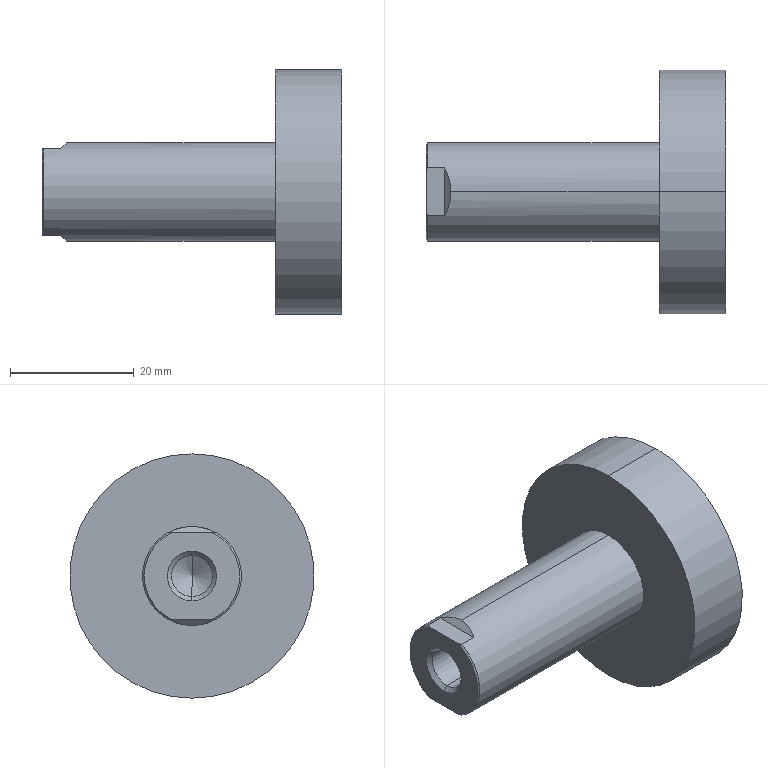Part | SolidWorks | features BaseBody 1 | 1 solid | 19 faces | box 48.5 x 39.5 x 39.5 mm | volume 20251 mm3 | plane 7 | cylinder 6 | cone 6 | commonest cylinder face diameters 6.647 x2 16 x2 39.5 x2
STEP:
#1=CARTESIAN_POINT('',(30.7,0.,8.));
#2=VERTEX_POINT('',#1);
#3=CARTESIAN_POINT('',(30.7,0.,-8.));
#4=VERTEX_POINT('',#3);
#5=CARTESIAN_POINT('',(30.7,0.,0.));
#6=DIRECTION('',(-1.,0.,0.));
#7=DIRECTION('',(0.,0.,1.));
#8=AXIS2_PLACEMENT_3D('',#5,#6,#7);
#9=CIRCLE('',#8,8.);
#10=EDGE_CURVE('',#2,#4,#9,.T.);
#11=ORIENTED_EDGE('',*,*,#10,.T.);
#12=CARTESIAN_POINT('',(-3.,0.,-8.));
#13=VERTEX_POINT('',#12);
#14=CARTESIAN_POINT('',(0.,0.,-8.));
#15=DIRECTION('',(-1.,0.,0.));
#16=VECTOR('',#15,1000.);
#17=LINE('',#14,#16);
#18=EDGE_CURVE('',#4,#13,#17,.T.);
#19=ORIENTED_EDGE('',*,*,#18,.T.);
#20=CARTESIAN_POINT('',(-4.,3.873,-7.));
#21=VERTEX_POINT('',#20);
#22=CARTESIAN_POINT('',(-3.,0.,-8.));
#23=CARTESIAN_POINT('',(-3.,1.362,-8.));
#24=CARTESIAN_POINT('',(-3.341,2.681,-7.659));
#25=CARTESIAN_POINT('',(-4.,3.873,-7.));
#26=(BOUNDED_CURVE()B_SPLINE_CURVE(3,(#22,#23,#24,#25),.UNSPECIFIED.,.F.,.F.)B_SPLINE_CURVE_WITH_KNOTS((4,4),(3.142,3.647),.UNSPECIFIED.)CURVE()GEOMETRIC_REPRESENTATION_ITEM()RATIONAL_B_SPLINE_CURVE((1.,0.9788,0.9788,1.))REPRESENTATION_ITEM(''));
#27=EDGE_CURVE('',#13,#21,#26,.T.);
#28=ORIENTED_EDGE('',*,*,#27,.T.);
#29=CARTESIAN_POINT('',(-6.75,3.873,-7.));
#30=VERTEX_POINT('',#29);
#31=CARTESIAN_POINT('',(0.,3.873,-7.));
#32=DIRECTION('',(-1.,0.,0.));
#33=VECTOR('',#32,1000.);
#34=LINE('',#31,#33);
#35=EDGE_CURVE('',#21,#30,#34,.T.);
#36=ORIENTED_EDGE('',*,*,#35,.T.);
#37=CARTESIAN_POINT('',(-6.75,3.873,7.));
#38=VERTEX_POINT('',#37);
#39=CARTESIAN_POINT('',(-6.75,0.,0.));
#40=DIRECTION('',(1.,0.,0.));
#41=DIRECTION('',(0.,0.,1.));
#42=AXIS2_PLACEMENT_3D('',#39,#40,#41);
#43=CIRCLE('',#42,8.);
#44=EDGE_CURVE('',#30,#38,#43,.T.);
#45=ORIENTED_EDGE('',*,*,#44,.T.);
#46=CARTESIAN_POINT('',(-4.,3.873,7.));
#47=VERTEX_POINT('',#46);
#48=CARTESIAN_POINT('',(0.,3.873,7.));
#49=DIRECTION('',(1.,0.,0.));
#50=VECTOR('',#49,1000.);
#51=LINE('',#48,#50);
#52=EDGE_CURVE('',#38,#47,#51,.T.);
#53=ORIENTED_EDGE('',*,*,#52,.T.);
#54=CARTESIAN_POINT('',(-3.,0.,8.));
#55=VERTEX_POINT('',#54);
#56=CARTESIAN_POINT('',(-4.,3.873,7.));
#57=CARTESIAN_POINT('',(-3.341,2.681,7.659));
#58=CARTESIAN_POINT('',(-3.,1.362,8.));
#59=CARTESIAN_POINT('',(-3.,0.,8.));
#60=(BOUNDED_CURVE()B_SPLINE_CURVE(3,(#56,#57,#58,#59),.UNSPECIFIED.,.F.,.F.)B_SPLINE_CURVE_WITH_KNOTS((4,4),(2.636,3.142),.UNSPECIFIED.)CURVE()GEOMETRIC_REPRESENTATION_ITEM()RATIONAL_B_SPLINE_CURVE((1.,0.9788,0.9788,1.))REPRESENTATION_ITEM(''));
#61=EDGE_CURVE('',#47,#55,#60,.T.);
#62=ORIENTED_EDGE('',*,*,#61,.T.);
#63=CARTESIAN_POINT('',(0.,0.,8.));
#64=DIRECTION('',(-1.,0.,0.));
#65=VECTOR('',#64,1000.);
#66=LINE('',#63,#65);
#67=EDGE_CURVE('',#2,#55,#66,.T.);
#68=ORIENTED_EDGE('',*,*,#67,.F.);
#69=EDGE_LOOP('',(#11,#19,#28,#36,#45,#53,#62,#68));
#70=FACE_OUTER_BOUND('',#69,.T.);
#71=CARTESIAN_POINT('',(0.,0.,0.));
#72=DIRECTION('',(-1.,0.,0.));
#73=DIRECTION('',(0.,0.,1.));
#74=AXIS2_PLACEMENT_3D('',#71,#72,#73);
#75=CYLINDRICAL_SURFACE('',#74,8.);
#76=ADVANCED_FACE('',(#70),#75,.T.);
#77=CARTESIAN_POINT('',(41.5,0.,19.75));
#78=VERTEX_POINT('',#77);
#79=CARTESIAN_POINT('',(41.5,0.,-19.75));
#80=VERTEX_POINT('',#79);
#81=CARTESIAN_POINT('',(41.5,0.,0.));
#82=DIRECTION('',(-1.,0.,0.));
#83=DIRECTION('',(0.,0.,1.));
#84=AXIS2_PLACEMENT_3D('',#81,#82,#83);
#85=CIRCLE('',#84,19.75);
#86=EDGE_CURVE('',#78,#80,#85,.T.);
#87=ORIENTED_EDGE('',*,*,#86,.T.);
#88=CARTESIAN_POINT('',(30.7,0.,-19.75));
#89=VERTEX_POINT('',#88);
#90=CARTESIAN_POINT('',(41.5,0.,-19.75));
#91=DIRECTION('',(-1.,0.,0.));
#92=VECTOR('',#91,1000.);
#93=LINE('',#90,#92);
#94=EDGE_CURVE('',#80,#89,#93,.T.);
#95=ORIENTED_EDGE('',*,*,#94,.T.);
#96=CARTESIAN_POINT('',(30.7,0.,19.75));
#97=VERTEX_POINT('',#96);
#98=CARTESIAN_POINT('',(30.7,0.,0.));
#99=DIRECTION('',(1.,0.,0.));
#100=DIRECTION('',(0.,0.,1.));
#101=AXIS2_PLACEMENT_3D('',#98,#99,#100);
#102=CIRCLE('',#101,19.75);
#103=EDGE_CURVE('',#89,#97,#102,.T.);
#104=ORIENTED_EDGE('',*,*,#103,.T.);
#105=CARTESIAN_POINT('',(41.5,0.,19.75));
#106=DIRECTION('',(-1.,0.,0.));
#107=VECTOR('',#106,1000.);
#108=LINE('',#105,#107);
#109=EDGE_CURVE('',#78,#97,#108,.T.);
#110=ORIENTED_EDGE('',*,*,#109,.F.);
#111=EDGE_LOOP('',(#87,#95,#104,#110));
#112=FACE_OUTER_BOUND('',#111,.T.);
#113=CARTESIAN_POINT('',(41.5,0.,0.));
#114=DIRECTION('',(-1.,0.,0.));
#115=DIRECTION('',(0.,0.,1.));
#116=AXIS2_PLACEMENT_3D('',#113,#114,#115);
#117=CYLINDRICAL_SURFACE('',#116,19.75);
#118=ADVANCED_FACE('',(#112),#117,.T.);
#119=CARTESIAN_POINT('',(-6.324,0.,-3.324));
#120=VERTEX_POINT('',#119);
#121=CARTESIAN_POINT('',(-6.324,0.,3.324));
#122=VERTEX_POINT('',#121);
#123=CARTESIAN_POINT('',(-6.324,0.,0.));
#124=DIRECTION('',(-1.,0.,0.));
#125=DIRECTION('',(0.,0.,1.));
#126=AXIS2_PLACEMENT_3D('',#123,#124,#125);
#127=CIRCLE('',#126,3.324);
#128=EDGE_CURVE('',#120,#122,#127,.T.);
#129=ORIENTED_EDGE('',*,*,#128,.F.);
#130=CARTESIAN_POINT('',(-7.,0.,-4.));
#131=VERTEX_POINT('',#130);
#132=CARTESIAN_POINT('',(-7.,0.,-4.));
#133=DIRECTION('',(-0.7071,0.,-0.7071));
#134=VECTOR('',#133,1000.);
#135=LINE('',#132,#134);
#136=EDGE_CURVE('',#120,#131,#135,.T.);
#137=ORIENTED_EDGE('',*,*,#136,.T.);
#138=CARTESIAN_POINT('',(-7.,0.,4.));
#139=VERTEX_POINT('',#138);
#140=CARTESIAN_POINT('',(-7.,0.,0.));
#141=DIRECTION('',(-1.,0.,0.));
#142=DIRECTION('',(0.,0.,1.));
#143=AXIS2_PLACEMENT_3D('',#140,#141,#142);
#144=CIRCLE('',#143,4.);
#145=EDGE_CURVE('',#131,#139,#144,.T.);
#146=ORIENTED_EDGE('',*,*,#145,.T.);
#147=CARTESIAN_POINT('',(-7.,0.,4.));
#148=DIRECTION('',(-0.7071,0.,0.7071));
#149=VECTOR('',#148,1000.);
#150=LINE('',#147,#149);
#151=EDGE_CURVE('',#122,#139,#150,.T.);
#152=ORIENTED_EDGE('',*,*,#151,.F.);
#153=EDGE_LOOP('',(#129,#137,#146,#152));
#154=FACE_OUTER_BOUND('',#153,.T.);
#155=CARTESIAN_POINT('',(-7.,0.,0.));
#156=DIRECTION('',(-1.,0.,0.));
#157=DIRECTION('',(0.,0.,1.));
#158=AXIS2_PLACEMENT_3D('',#155,#156,#157);
#159=CONICAL_SURFACE('',#158,4.,0.7854);
#160=ADVANCED_FACE('',(#154),#159,.F.);
#161=CARTESIAN_POINT('',(7.4,0.,-3.323));
#162=VERTEX_POINT('',#161);
#163=CARTESIAN_POINT('',(7.4,0.,3.323));
#164=VERTEX_POINT('',#163);
#165=CARTESIAN_POINT('',(7.4,0.,0.));
#166=DIRECTION('',(-1.,0.,0.));
#167=DIRECTION('',(0.,0.,1.));
#168=AXIS2_PLACEMENT_3D('',#165,#166,#167);
#169=CIRCLE('',#168,3.324);
#170=EDGE_CURVE('',#162,#164,#169,.T.);
#171=ORIENTED_EDGE('',*,*,#170,.F.);
#172=CARTESIAN_POINT('',(9.319,0.,-3.324));
#173=DIRECTION('',(-1.,0.,0.));
#174=VECTOR('',#173,1000.);
#175=LINE('',#172,#174);
#176=EDGE_CURVE('',#162,#120,#175,.T.);
#177=ORIENTED_EDGE('',*,*,#176,.T.);
#178=ORIENTED_EDGE('',*,*,#128,.T.);
#179=CARTESIAN_POINT('',(9.319,0.,3.324));
#180=DIRECTION('',(-1.,0.,0.));
#181=VECTOR('',#180,1000.);
#182=LINE('',#179,#181);
#183=EDGE_CURVE('',#164,#122,#182,.T.);
#184=ORIENTED_EDGE('',*,*,#183,.F.);
#185=EDGE_LOOP('',(#171,#177,#178,#184));
#186=FACE_OUTER_BOUND('',#185,.T.);
#187=CARTESIAN_POINT('',(9.319,0.,0.));
#188=DIRECTION('',(-1.,0.,0.));
#189=DIRECTION('',(0.,0.,1.));
#190=AXIS2_PLACEMENT_3D('',#187,#188,#189);
#191=CYLINDRICAL_SURFACE('',#190,3.324);
#192=ADVANCED_FACE('',(#186),#191,.F.);
#193=CARTESIAN_POINT('',(9.319,0.,0.));
#194=VERTEX_POINT('',#193);
#195=CARTESIAN_POINT('',(7.4,0.,3.323));
#196=DIRECTION('',(-0.5,0.,0.866));
#197=VECTOR('',#196,1000.);
#198=LINE('',#195,#197);
#199=EDGE_CURVE('',#194,#164,#198,.T.);
#200=ORIENTED_EDGE('',*,*,#199,.F.);
#201=CARTESIAN_POINT('',(7.4,0.,-3.323));
#202=DIRECTION('',(-0.5,0.,-0.866));
#203=VECTOR('',#202,1000.);
#204=LINE('',#201,#203);
#205=EDGE_CURVE('',#194,#162,#204,.T.);
#206=ORIENTED_EDGE('',*,*,#205,.T.);
#207=ORIENTED_EDGE('',*,*,#170,.T.);
#208=EDGE_LOOP('',(#200,#206,#207));
#209=FACE_OUTER_BOUND('',#208,.T.);
#210=CARTESIAN_POINT('',(7.4,0.,0.));
#211=DIRECTION('',(-1.,0.,0.));
#212=DIRECTION('',(0.,0.,1.));
#213=AXIS2_PLACEMENT_3D('',#210,#211,#212);
#214=CONICAL_SURFACE('',#213,3.323,1.047);
#215=ADVANCED_FACE('',(#209),#214,.F.);
#216=ORIENTED_EDGE('',*,*,#18,.F.);
#217=CARTESIAN_POINT('',(30.7,0.,0.));
#218=DIRECTION('',(-1.,0.,0.));
#219=DIRECTION('',(0.,0.,1.));
#220=AXIS2_PLACEMENT_3D('',#217,#218,#219);
#221=CIRCLE('',#220,8.);
#222=EDGE_CURVE('',#4,#2,#221,.T.);
#223=ORIENTED_EDGE('',*,*,#222,.T.);
#224=ORIENTED_EDGE('',*,*,#67,.T.);
#225=CARTESIAN_POINT('',(-4.,-3.873,7.));
#226=VERTEX_POINT('',#225);
#227=CARTESIAN_POINT('',(-3.,0.,8.));
#228=CARTESIAN_POINT('',(-3.,-1.362,8.));
#229=CARTESIAN_POINT('',(-3.341,-2.681,7.659));
#230=CARTESIAN_POINT('',(-4.,-3.873,7.));
#231=(BOUNDED_CURVE()B_SPLINE_CURVE(3,(#227,#228,#229,#230),.UNSPECIFIED.,.F.,.F.)B_SPLINE_CURVE_WITH_KNOTS((4,4),(3.142,3.647),.UNSPECIFIED.)CURVE()GEOMETRIC_REPRESENTATION_ITEM()RATIONAL_B_SPLINE_CURVE((1.,0.9788,0.9788,1.))REPRESENTATION_ITEM(''));
#232=EDGE_CURVE('',#55,#226,#231,.T.);
#233=ORIENTED_EDGE('',*,*,#232,.T.);
#234=CARTESIAN_POINT('',(-6.75,-3.873,7.));
#235=VERTEX_POINT('',#234);
#236=CARTESIAN_POINT('',(0.,-3.873,7.));
#237=DIRECTION('',(-1.,0.,0.));
#238=VECTOR('',#237,1000.);
#239=LINE('',#236,#238);
#240=EDGE_CURVE('',#226,#235,#239,.T.);
#241=ORIENTED_EDGE('',*,*,#240,.T.);
#242=CARTESIAN_POINT('',(-6.75,-3.873,-7.));
#243=VERTEX_POINT('',#242);
#244=CARTESIAN_POINT('',(-6.75,0.,0.));
#245=DIRECTION('',(1.,0.,0.));
#246=DIRECTION('',(0.,0.,1.));
#247=AXIS2_PLACEMENT_3D('',#244,#245,#246);
#248=CIRCLE('',#247,8.);
#249=EDGE_CURVE('',#235,#243,#248,.T.);
#250=ORIENTED_EDGE('',*,*,#249,.T.);
#251=CARTESIAN_POINT('',(-4.,-3.873,-7.));
#252=VERTEX_POINT('',#251);
#253=CARTESIAN_POINT('',(0.,-3.873,-7.));
#254=DIRECTION('',(1.,0.,0.));
#255=VECTOR('',#254,1000.);
#256=LINE('',#253,#255);
#257=EDGE_CURVE('',#243,#252,#256,.T.);
#258=ORIENTED_EDGE('',*,*,#257,.T.);
#259=CARTESIAN_POINT('',(-4.,-3.873,-7.));
#260=CARTESIAN_POINT('',(-3.341,-2.681,-7.659));
#261=CARTESIAN_POINT('',(-3.,-1.362,-8.));
#262=CARTESIAN_POINT('',(-3.,0.,-8.));
#263=(BOUNDED_CURVE()B_SPLINE_CURVE(3,(#259,#260,#261,#262),.UNSPECIFIED.,.F.,.F.)B_SPLINE_CURVE_WITH_KNOTS((4,4),(2.636,3.142),.UNSPECIFIED.)CURVE()GEOMETRIC_REPRESENTATION_ITEM()RATIONAL_B_SPLINE_CURVE((1.,0.9788,0.9788,1.))REPRESENTATION_ITEM(''));
#264=EDGE_CURVE('',#252,#13,#263,.T.);
#265=ORIENTED_EDGE('',*,*,#264,.T.);
#266=EDGE_LOOP('',(#216,#223,#224,#233,#241,#250,#258,#265));
#267=FACE_OUTER_BOUND('',#266,.T.);
#268=CARTESIAN_POINT('',(0.,0.,0.));
#269=DIRECTION('',(-1.,0.,0.));
#270=DIRECTION('',(0.,0.,1.));
#271=AXIS2_PLACEMENT_3D('',#268,#269,#270);
#272=CYLINDRICAL_SURFACE('',#271,8.);
#273=ADVANCED_FACE('',(#267),#272,.T.);
#274=ORIENTED_EDGE('',*,*,#61,.F.);
#275=CARTESIAN_POINT('',(-4.,14.,7.));
#276=DIRECTION('',(0.,-1.,0.));
#277=VECTOR('',#276,1000.);
#278=LINE('',#275,#277);
#279=EDGE_CURVE('',#47,#226,#278,.T.);
#280=ORIENTED_EDGE('',*,*,#279,.T.);
#281=ORIENTED_EDGE('',*,*,#232,.F.);
#282=EDGE_LOOP('',(#274,#280,#281));
#283=FACE_OUTER_BOUND('',#282,.T.);
#284=CARTESIAN_POINT('',(1.,14.,12.));
#285=DIRECTION('',(-0.7071,0.,0.7071));
#286=DIRECTION('',(0.7071,0.,0.7071));
#287=AXIS2_PLACEMENT_3D('',#284,#285,#286);
#288=PLANE('',#287);
#289=ADVANCED_FACE('',(#283),#288,.T.);
#290=CARTESIAN_POINT('',(-7.,3.326,7.));
#291=VERTEX_POINT('',#290);
#292=CARTESIAN_POINT('',(-6.75,3.873,7.));
#293=CARTESIAN_POINT('',(-6.84,3.688,7.));
#294=CARTESIAN_POINT('',(-6.923,3.505,7.));
#295=CARTESIAN_POINT('',(-7.,3.326,7.));
#296=B_SPLINE_CURVE_WITH_KNOTS('',3,(#292,#293,#294,#295),.UNSPECIFIED.,.F.,.F.,(4,4),(0.,1.),.UNSPECIFIED.);
#297=EDGE_CURVE('',#38,#291,#296,.T.);
#298=ORIENTED_EDGE('',*,*,#297,.T.);
#299=CARTESIAN_POINT('',(-7.,-3.326,7.));
#300=VERTEX_POINT('',#299);
#301=CARTESIAN_POINT('',(-7.,14.,7.));
#302=DIRECTION('',(0.,-1.,0.));
#303=VECTOR('',#302,1000.);
#304=LINE('',#301,#303);
#305=EDGE_CURVE('',#291,#300,#304,.T.);
#306=ORIENTED_EDGE('',*,*,#305,.T.);
#307=CARTESIAN_POINT('',(-7.,-3.326,7.));
#308=CARTESIAN_POINT('',(-6.923,-3.505,7.));
#309=CARTESIAN_POINT('',(-6.84,-3.688,7.));
#310=CARTESIAN_POINT('',(-6.75,-3.873,7.));
#311=B_SPLINE_CURVE_WITH_KNOTS('',3,(#307,#308,#309,#310),.UNSPECIFIED.,.F.,.F.,(4,4),(0.,1.),.UNSPECIFIED.);
#312=EDGE_CURVE('',#300,#235,#311,.T.);
#313=ORIENTED_EDGE('',*,*,#312,.T.);
#314=ORIENTED_EDGE('',*,*,#240,.F.);
#315=ORIENTED_EDGE('',*,*,#279,.F.);
#316=ORIENTED_EDGE('',*,*,#52,.F.);
#317=EDGE_LOOP('',(#298,#306,#313,#314,#315,#316));
#318=FACE_OUTER_BOUND('',#317,.T.);
#319=CARTESIAN_POINT('',(-4.,14.,7.));
#320=DIRECTION('',(0.,0.,1.));
#321=DIRECTION('',(1.,0.,0.));
#322=AXIS2_PLACEMENT_3D('',#319,#320,#321);
#323=PLANE('',#322);
#324=ADVANCED_FACE('',(#318),#323,.T.);
#325=ORIENTED_EDGE('',*,*,#297,.F.);
#326=ORIENTED_EDGE('',*,*,#44,.F.);
#327=CARTESIAN_POINT('',(-7.,3.326,-7.));
#328=VERTEX_POINT('',#327);
#329=CARTESIAN_POINT('',(-6.75,3.873,-7.));
#330=CARTESIAN_POINT('',(-6.839,3.689,-7.));
#331=CARTESIAN_POINT('',(-6.922,3.507,-7.));
#332=CARTESIAN_POINT('',(-7.,3.326,-7.));
#333=B_SPLINE_CURVE_WITH_KNOTS('',3,(#329,#330,#331,#332),.UNSPECIFIED.,.F.,.F.,(4,4),(0.,1.),.UNSPECIFIED.);
#334=EDGE_CURVE('',#30,#328,#333,.T.);
#335=ORIENTED_EDGE('',*,*,#334,.T.);
#336=CARTESIAN_POINT('',(-7.,0.,0.));
#337=DIRECTION('',(1.,0.,0.));
#338=DIRECTION('',(0.,0.,-1.));
#339=AXIS2_PLACEMENT_3D('',#336,#337,#338);
#340=CIRCLE('',#339,7.75);
#341=EDGE_CURVE('',#328,#291,#340,.T.);
#342=ORIENTED_EDGE('',*,*,#341,.T.);
#343=EDGE_LOOP('',(#325,#326,#335,#342));
#344=FACE_OUTER_BOUND('',#343,.T.);
#345=CARTESIAN_POINT('',(-6.75,0.,0.));
#346=DIRECTION('',(1.,0.,0.));
#347=DIRECTION('',(0.,0.,-1.));
#348=AXIS2_PLACEMENT_3D('',#345,#346,#347);
#349=CONICAL_SURFACE('',#348,8.,0.7854);
#350=ADVANCED_FACE('',(#344),#349,.T.);
#351=CARTESIAN_POINT('',(-7.,-3.326,-7.));
#352=VERTEX_POINT('',#351);
#353=CARTESIAN_POINT('',(-6.75,-3.873,-7.));
#354=CARTESIAN_POINT('',(-6.84,-3.688,-7.));
#355=CARTESIAN_POINT('',(-6.923,-3.505,-7.));
#356=CARTESIAN_POINT('',(-7.,-3.326,-7.));
#357=B_SPLINE_CURVE_WITH_KNOTS('',3,(#353,#354,#355,#356),.UNSPECIFIED.,.F.,.F.,(4,4),(0.,1.),.UNSPECIFIED.);
#358=EDGE_CURVE('',#243,#352,#357,.T.);
#359=ORIENTED_EDGE('',*,*,#358,.T.);
#360=CARTESIAN_POINT('',(-7.,14.,-7.));
#361=DIRECTION('',(0.,1.,0.));
#362=VECTOR('',#361,1000.);
#363=LINE('',#360,#362);
#364=EDGE_CURVE('',#352,#328,#363,.T.);
#365=ORIENTED_EDGE('',*,*,#364,.T.);
#366=ORIENTED_EDGE('',*,*,#334,.F.);
#367=ORIENTED_EDGE('',*,*,#35,.F.);
#368=CARTESIAN_POINT('',(-4.,14.,-7.));
#369=DIRECTION('',(0.,-1.,0.));
#370=VECTOR('',#369,1000.);
#371=LINE('',#368,#370);
#372=EDGE_CURVE('',#21,#252,#371,.T.);
#373=ORIENTED_EDGE('',*,*,#372,.T.);
#374=ORIENTED_EDGE('',*,*,#257,.F.);
#375=EDGE_LOOP('',(#359,#365,#366,#367,#373,#374));
#376=FACE_OUTER_BOUND('',#375,.T.);
#377=CARTESIAN_POINT('',(-7.,14.,-7.));
#378=DIRECTION('',(0.,0.,-1.));
#379=DIRECTION('',(-1.,0.,0.));
#380=AXIS2_PLACEMENT_3D('',#377,#378,#379);
#381=PLANE('',#380);
#382=ADVANCED_FACE('',(#376),#381,.T.);
#383=ORIENTED_EDGE('',*,*,#264,.F.);
#384=ORIENTED_EDGE('',*,*,#372,.F.);
#385=ORIENTED_EDGE('',*,*,#27,.F.);
#386=EDGE_LOOP('',(#383,#384,#385));
#387=FACE_OUTER_BOUND('',#386,.T.);
#388=CARTESIAN_POINT('',(-4.,14.,-7.));
#389=DIRECTION('',(-0.7071,0.,-0.7071));
#390=DIRECTION('',(-0.7071,0.,0.7071));
#391=AXIS2_PLACEMENT_3D('',#388,#389,#390);
#392=PLANE('',#391);
#393=ADVANCED_FACE('',(#387),#392,.T.);
#394=ORIENTED_EDGE('',*,*,#358,.F.);
#395=ORIENTED_EDGE('',*,*,#249,.F.);
#396=ORIENTED_EDGE('',*,*,#312,.F.);
#397=CARTESIAN_POINT('',(-7.,0.,0.));
#398=DIRECTION('',(1.,0.,0.));
#399=DIRECTION('',(0.,0.,-1.));
#400=AXIS2_PLACEMENT_3D('',#397,#398,#399);
#401=CIRCLE('',#400,7.75);
#402=EDGE_CURVE('',#300,#352,#401,.T.);
#403=ORIENTED_EDGE('',*,*,#402,.T.);
#404=EDGE_LOOP('',(#394,#395,#396,#403));
#405=FACE_OUTER_BOUND('',#404,.T.);
#406=CARTESIAN_POINT('',(-6.75,0.,0.));
#407=DIRECTION('',(1.,0.,0.));
#408=DIRECTION('',(0.,0.,-1.));
#409=AXIS2_PLACEMENT_3D('',#406,#407,#408);
#410=CONICAL_SURFACE('',#409,8.,0.7854);
#411=ADVANCED_FACE('',(#405),#410,.T.);
#412=ORIENTED_EDGE('',*,*,#10,.F.);
#413=ORIENTED_EDGE('',*,*,#222,.F.);
#414=EDGE_LOOP('',(#412,#413));
#415=FACE_BOUND('',#414,.T.);
#416=CARTESIAN_POINT('',(30.7,0.,0.));
#417=DIRECTION('',(1.,0.,0.));
#418=DIRECTION('',(0.,0.,1.));
#419=AXIS2_PLACEMENT_3D('',#416,#417,#418);
#420=CIRCLE('',#419,19.75);
#421=EDGE_CURVE('',#97,#89,#420,.T.);
#422=ORIENTED_EDGE('',*,*,#421,.F.);
#423=ORIENTED_EDGE('',*,*,#103,.F.);
#424=EDGE_LOOP('',(#422,#423));
#425=FACE_OUTER_BOUND('',#424,.T.);
#426=CARTESIAN_POINT('',(30.7,8.,0.));
#427=DIRECTION('',(1.,0.,0.));
#428=DIRECTION('',(0.,0.,-1.));
#429=AXIS2_PLACEMENT_3D('',#426,#427,#428);
#430=PLANE('',#429);
#431=ADVANCED_FACE('',(#415,#425),#430,.F.);
#432=CARTESIAN_POINT('',(-7.,0.,0.));
#433=DIRECTION('',(-1.,0.,0.));
#434=DIRECTION('',(0.,0.,1.));
#435=AXIS2_PLACEMENT_3D('',#432,#433,#434);
#436=CIRCLE('',#435,4.);
#437=EDGE_CURVE('',#139,#131,#436,.T.);
#438=ORIENTED_EDGE('',*,*,#437,.F.);
#439=ORIENTED_EDGE('',*,*,#145,.F.);
#440=EDGE_LOOP('',(#438,#439));
#441=FACE_BOUND('',#440,.T.);
#442=ORIENTED_EDGE('',*,*,#364,.F.);
#443=ORIENTED_EDGE('',*,*,#402,.F.);
#444=ORIENTED_EDGE('',*,*,#305,.F.);
#445=ORIENTED_EDGE('',*,*,#341,.F.);
#446=EDGE_LOOP('',(#442,#443,#444,#445));
#447=FACE_OUTER_BOUND('',#446,.T.);
#448=CARTESIAN_POINT('',(-7.,0.,0.));
#449=DIRECTION('',(1.,0.,0.));
#450=DIRECTION('',(0.,0.,-1.));
#451=AXIS2_PLACEMENT_3D('',#448,#449,#450);
#452=PLANE('',#451);
#453=ADVANCED_FACE('',(#441,#447),#452,.F.);
#454=ORIENTED_EDGE('',*,*,#94,.F.);
#455=CARTESIAN_POINT('',(41.5,0.,0.));
#456=DIRECTION('',(-1.,0.,0.));
#457=DIRECTION('',(0.,0.,1.));
#458=AXIS2_PLACEMENT_3D('',#455,#456,#457);
#459=CIRCLE('',#458,19.75);
#460=EDGE_CURVE('',#80,#78,#459,.T.);
#461=ORIENTED_EDGE('',*,*,#460,.T.);
#462=ORIENTED_EDGE('',*,*,#109,.T.);
#463=ORIENTED_EDGE('',*,*,#421,.T.);
#464=EDGE_LOOP('',(#454,#461,#462,#463));
#465=FACE_OUTER_BOUND('',#464,.T.);
#466=CARTESIAN_POINT('',(41.5,0.,0.));
#467=DIRECTION('',(-1.,0.,0.));
#468=DIRECTION('',(0.,0.,1.));
#469=AXIS2_PLACEMENT_3D('',#466,#467,#468);
#470=CYLINDRICAL_SURFACE('',#469,19.75);
#471=ADVANCED_FACE('',(#465),#470,.T.);
#472=ORIENTED_EDGE('',*,*,#136,.F.);
#473=CARTESIAN_POINT('',(-6.324,0.,0.));
#474=DIRECTION('',(-1.,0.,0.));
#475=DIRECTION('',(0.,0.,1.));
#476=AXIS2_PLACEMENT_3D('',#473,#474,#475);
#477=CIRCLE('',#476,3.324);
#478=EDGE_CURVE('',#122,#120,#477,.T.);
#479=ORIENTED_EDGE('',*,*,#478,.F.);
#480=ORIENTED_EDGE('',*,*,#151,.T.);
#481=ORIENTED_EDGE('',*,*,#437,.T.);
#482=EDGE_LOOP('',(#472,#479,#480,#481));
#483=FACE_OUTER_BOUND('',#482,.T.);
#484=CARTESIAN_POINT('',(-7.,0.,0.));
#485=DIRECTION('',(-1.,0.,0.));
#486=DIRECTION('',(0.,0.,1.));
#487=AXIS2_PLACEMENT_3D('',#484,#485,#486);
#488=CONICAL_SURFACE('',#487,4.,0.7854);
#489=ADVANCED_FACE('',(#483),#488,.F.);
#490=ORIENTED_EDGE('',*,*,#86,.F.);
#491=ORIENTED_EDGE('',*,*,#460,.F.);
#492=EDGE_LOOP('',(#490,#491));
#493=FACE_OUTER_BOUND('',#492,.T.);
#494=CARTESIAN_POINT('',(41.5,19.75,0.));
#495=DIRECTION('',(-1.,0.,0.));
#496=DIRECTION('',(0.,0.,1.));
#497=AXIS2_PLACEMENT_3D('',#494,#495,#496);
#498=PLANE('',#497);
#499=ADVANCED_FACE('',(#493),#498,.F.);
#500=ORIENTED_EDGE('',*,*,#176,.F.);
#501=CARTESIAN_POINT('',(7.4,0.,0.));
#502=DIRECTION('',(-1.,0.,0.));
#503=DIRECTION('',(0.,0.,1.));
#504=AXIS2_PLACEMENT_3D('',#501,#502,#503);
#505=CIRCLE('',#504,3.324);
#506=EDGE_CURVE('',#164,#162,#505,.T.);
#507=ORIENTED_EDGE('',*,*,#506,.F.);
#508=ORIENTED_EDGE('',*,*,#183,.T.);
#509=ORIENTED_EDGE('',*,*,#478,.T.);
#510=EDGE_LOOP('',(#500,#507,#508,#509));
#511=FACE_OUTER_BOUND('',#510,.T.);
#512=CARTESIAN_POINT('',(9.319,0.,0.));
#513=DIRECTION('',(-1.,0.,0.));
#514=DIRECTION('',(0.,0.,1.));
#515=AXIS2_PLACEMENT_3D('',#512,#513,#514);
#516=CYLINDRICAL_SURFACE('',#515,3.324);
#517=ADVANCED_FACE('',(#511),#516,.F.);
#518=ORIENTED_EDGE('',*,*,#205,.F.);
#519=ORIENTED_EDGE('',*,*,#199,.T.);
#520=ORIENTED_EDGE('',*,*,#506,.T.);
#521=EDGE_LOOP('',(#518,#519,#520));
#522=FACE_OUTER_BOUND('',#521,.T.);
#523=CARTESIAN_POINT('',(7.4,0.,0.));
#524=DIRECTION('',(-1.,0.,0.));
#525=DIRECTION('',(0.,0.,1.));
#526=AXIS2_PLACEMENT_3D('',#523,#524,#525);
#527=CONICAL_SURFACE('',#526,3.323,1.047);
#528=ADVANCED_FACE('',(#522),#527,.F.);
#529=CLOSED_SHELL('',(#76,#118,#160,#192,#215,#273,#289,#324,#350,#382,#393,#411,#431,#453,#471,#489,#499,#517,#528));
#530=MANIFOLD_SOLID_BREP('',#529);
#531=CARTESIAN_POINT('',(0.,0.,0.));
#532=DIRECTION('',(0.,0.,1.));
#533=DIRECTION('',(1.,0.,0.));
#534=AXIS2_PLACEMENT_3D('',#531,#532,#533);
#535=(LENGTH_UNIT()NAMED_UNIT(*)SI_UNIT(.MILLI.,.METRE.));
#536=UNCERTAINTY_MEASURE_WITH_UNIT(LENGTH_MEASURE(0.00001),#535,'','');
#537=(NAMED_UNIT(*)PLANE_ANGLE_UNIT()SI_UNIT($,.RADIAN.));
#538=(NAMED_UNIT(*)SI_UNIT($,.STERADIAN.)SOLID_ANGLE_UNIT());
#539=(GEOMETRIC_REPRESENTATION_CONTEXT(3)GLOBAL_UNCERTAINTY_ASSIGNED_CONTEXT((#536))GLOBAL_UNIT_ASSIGNED_CONTEXT((#535,#537,#538))REPRESENTATION_CONTEXT('',''));
#540=ADVANCED_BREP_SHAPE_REPRESENTATION('',(#530,#534),#539);